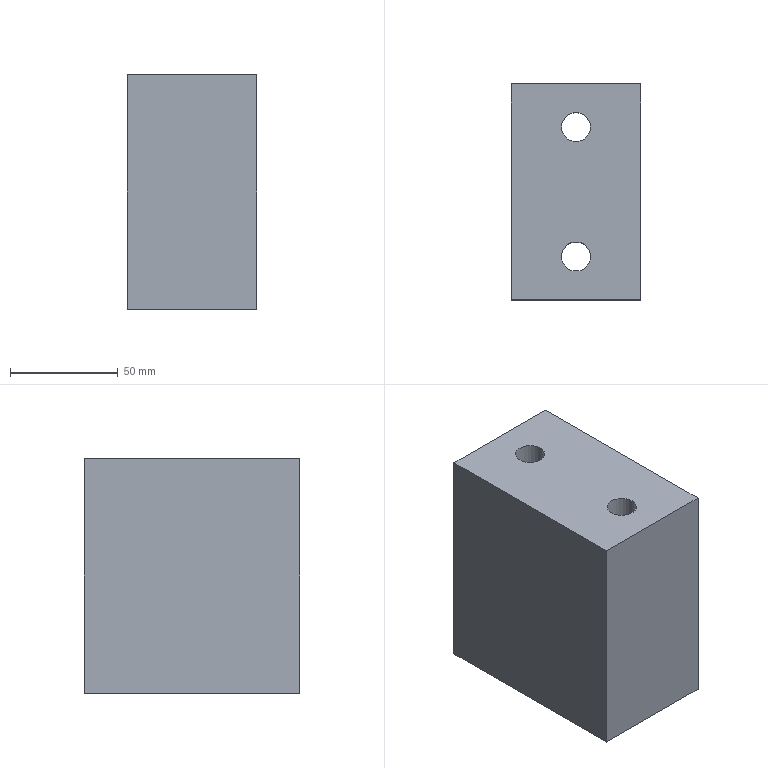Part | NX | features 15 2 | 1 solid | 12 faces | box 60 x 100 x 108.5 mm | volume 596509 mm3 | plane 8 | cylinder 4 | commonest cylinder face diameters 13.5 x2 20 x2
STEP:
#1=CARTESIAN_POINT('',(3961.75,-592.5,61.));
#2=VERTEX_POINT('',#1);
#3=CARTESIAN_POINT('',(3955.,-592.5,61.));
#4=DIRECTION('',(0.,0.,1.));
#5=DIRECTION('',(1.,0.,0.));
#6=AXIS2_PLACEMENT_3D('',#3,#4,#5);
#7=CIRCLE('',#6,6.75);
#8=EDGE_CURVE('',#2,#2,#7,.T.);
#9=ORIENTED_EDGE('',*,*,#8,.T.);
#10=EDGE_LOOP('',(#9));
#11=FACE_BOUND('',#10,.T.);
#12=CARTESIAN_POINT('',(3955.,-602.5,61.));
#13=VERTEX_POINT('',#12);
#14=CARTESIAN_POINT('',(3955.,-592.5,61.));
#15=DIRECTION('',(0.,0.,1.));
#16=DIRECTION('',(0.,-1.,0.));
#17=AXIS2_PLACEMENT_3D('',#14,#15,#16);
#18=CIRCLE('',#17,10.);
#19=EDGE_CURVE('',#13,#13,#18,.T.);
#20=ORIENTED_EDGE('',*,*,#19,.F.);
#21=EDGE_LOOP('',(#20));
#22=FACE_BOUND('',#21,.T.);
#23=CARTESIAN_POINT('',(3959.241,-596.363,61.));
#24=DIRECTION('',(0.,0.,1.));
#25=DIRECTION('',(0.,-1.,0.));
#26=AXIS2_PLACEMENT_3D('',#23,#24,#25);
#27=PLANE('',#26);
#28=ADVANCED_FACE('',(#11,#22),#27,.F.);
#29=ORIENTED_EDGE('',*,*,#19,.T.);
#30=EDGE_LOOP('',(#29));
#31=FACE_BOUND('',#30,.T.);
#32=CARTESIAN_POINT('',(3955.,-602.5,-7.5));
#33=VERTEX_POINT('',#32);
#34=CARTESIAN_POINT('',(3955.,-592.5,-7.5));
#35=DIRECTION('',(0.,0.,-1.));
#36=DIRECTION('',(0.,-1.,0.));
#37=AXIS2_PLACEMENT_3D('',#34,#35,#36);
#38=CIRCLE('',#37,10.);
#39=EDGE_CURVE('',#33,#33,#38,.T.);
#40=ORIENTED_EDGE('',*,*,#39,.T.);
#41=EDGE_LOOP('',(#40));
#42=FACE_BOUND('',#41,.T.);
#43=CARTESIAN_POINT('',(3955.,-592.5,-7.5));
#44=DIRECTION('',(0.,0.,1.));
#45=DIRECTION('',(0.,-1.,0.));
#46=AXIS2_PLACEMENT_3D('',#43,#44,#45);
#47=CYLINDRICAL_SURFACE('',#46,10.);
#48=ADVANCED_FACE('',(#31,#42),#47,.F.);
#49=CARTESIAN_POINT('',(3961.75,-592.5,101.));
#50=VERTEX_POINT('',#49);
#51=CARTESIAN_POINT('',(3955.,-592.5,101.));
#52=DIRECTION('',(0.,0.,1.));
#53=DIRECTION('',(1.,0.,0.));
#54=AXIS2_PLACEMENT_3D('',#51,#52,#53);
#55=CIRCLE('',#54,6.75);
#56=EDGE_CURVE('',#50,#50,#55,.T.);
#57=ORIENTED_EDGE('',*,*,#56,.T.);
#58=EDGE_LOOP('',(#57));
#59=FACE_BOUND('',#58,.T.);
#60=ORIENTED_EDGE('',*,*,#8,.F.);
#61=EDGE_LOOP('',(#60));
#62=FACE_BOUND('',#61,.T.);
#63=CARTESIAN_POINT('',(3955.,-592.5,12.5));
#64=DIRECTION('',(0.,0.,1.));
#65=DIRECTION('',(0.,-1.,0.));
#66=AXIS2_PLACEMENT_3D('',#63,#64,#65);
#67=CYLINDRICAL_SURFACE('',#66,6.75);
#68=ADVANCED_FACE('',(#59,#62),#67,.F.);
#69=CARTESIAN_POINT('',(3961.75,-652.5,61.));
#70=VERTEX_POINT('',#69);
#71=CARTESIAN_POINT('',(3955.,-652.5,61.));
#72=DIRECTION('',(0.,0.,1.));
#73=DIRECTION('',(1.,0.,0.));
#74=AXIS2_PLACEMENT_3D('',#71,#72,#73);
#75=CIRCLE('',#74,6.75);
#76=EDGE_CURVE('',#70,#70,#75,.T.);
#77=ORIENTED_EDGE('',*,*,#76,.T.);
#78=EDGE_LOOP('',(#77));
#79=FACE_BOUND('',#78,.T.);
#80=CARTESIAN_POINT('',(3955.,-662.5,61.));
#81=VERTEX_POINT('',#80);
#82=CARTESIAN_POINT('',(3955.,-652.5,61.));
#83=DIRECTION('',(0.,0.,1.));
#84=DIRECTION('',(0.,-1.,0.));
#85=AXIS2_PLACEMENT_3D('',#82,#83,#84);
#86=CIRCLE('',#85,10.);
#87=EDGE_CURVE('',#81,#81,#86,.T.);
#88=ORIENTED_EDGE('',*,*,#87,.F.);
#89=EDGE_LOOP('',(#88));
#90=FACE_BOUND('',#89,.T.);
#91=CARTESIAN_POINT('',(3959.241,-648.637,61.));
#92=DIRECTION('',(0.,0.,1.));
#93=DIRECTION('',(0.,1.,0.));
#94=AXIS2_PLACEMENT_3D('',#91,#92,#93);
#95=PLANE('',#94);
#96=ADVANCED_FACE('',(#79,#90),#95,.F.);
#97=CARTESIAN_POINT('',(3961.75,-652.5,101.));
#98=VERTEX_POINT('',#97);
#99=CARTESIAN_POINT('',(3955.,-652.5,101.));
#100=DIRECTION('',(0.,0.,1.));
#101=DIRECTION('',(1.,0.,0.));
#102=AXIS2_PLACEMENT_3D('',#99,#100,#101);
#103=CIRCLE('',#102,6.75);
#104=EDGE_CURVE('',#98,#98,#103,.T.);
#105=ORIENTED_EDGE('',*,*,#104,.T.);
#106=EDGE_LOOP('',(#105));
#107=FACE_BOUND('',#106,.T.);
#108=ORIENTED_EDGE('',*,*,#76,.F.);
#109=EDGE_LOOP('',(#108));
#110=FACE_BOUND('',#109,.T.);
#111=CARTESIAN_POINT('',(3955.,-652.5,12.5));
#112=DIRECTION('',(0.,0.,1.));
#113=DIRECTION('',(0.,1.,0.));
#114=AXIS2_PLACEMENT_3D('',#111,#112,#113);
#115=CYLINDRICAL_SURFACE('',#114,6.75);
#116=ADVANCED_FACE('',(#107,#110),#115,.F.);
#117=CARTESIAN_POINT('',(3925.,-572.5,101.));
#118=VERTEX_POINT('',#117);
#119=CARTESIAN_POINT('',(3925.,-572.5,-7.5));
#120=VERTEX_POINT('',#119);
#121=CARTESIAN_POINT('',(3925.,-572.5,48.));
#122=DIRECTION('',(0.,0.,-1.));
#123=VECTOR('',#122,1000.);
#124=LINE('',#121,#123);
#125=EDGE_CURVE('',#118,#120,#124,.T.);
#126=ORIENTED_EDGE('',*,*,#125,.F.);
#127=CARTESIAN_POINT('',(3985.,-572.5,101.));
#128=VERTEX_POINT('',#127);
#129=CARTESIAN_POINT('',(3985.,-572.5,101.));
#130=DIRECTION('',(-1.,0.,0.));
#131=VECTOR('',#130,1000.);
#132=LINE('',#129,#131);
#133=EDGE_CURVE('',#128,#118,#132,.T.);
#134=ORIENTED_EDGE('',*,*,#133,.F.);
#135=CARTESIAN_POINT('',(3985.,-572.5,-7.5));
#136=VERTEX_POINT('',#135);
#137=CARTESIAN_POINT('',(3985.,-572.5,48.));
#138=DIRECTION('',(0.,0.,1.));
#139=VECTOR('',#138,1000.);
#140=LINE('',#137,#139);
#141=EDGE_CURVE('',#136,#128,#140,.T.);
#142=ORIENTED_EDGE('',*,*,#141,.F.);
#143=CARTESIAN_POINT('',(3985.,-572.5,-7.5));
#144=DIRECTION('',(1.,0.,0.));
#145=VECTOR('',#144,1000.);
#146=LINE('',#143,#145);
#147=EDGE_CURVE('',#120,#136,#146,.T.);
#148=ORIENTED_EDGE('',*,*,#147,.F.);
#149=EDGE_LOOP('',(#126,#134,#142,#148));
#150=FACE_BOUND('',#149,.T.);
#151=CARTESIAN_POINT('',(3985.,-572.5,48.));
#152=DIRECTION('',(0.,1.,0.));
#153=DIRECTION('',(0.,0.,-1.));
#154=AXIS2_PLACEMENT_3D('',#151,#152,#153);
#155=PLANE('',#154);
#156=ADVANCED_FACE('',(#150),#155,.T.);
#157=ORIENTED_EDGE('',*,*,#141,.T.);
#158=CARTESIAN_POINT('',(3985.,-672.5,101.));
#159=VERTEX_POINT('',#158);
#160=CARTESIAN_POINT('',(3985.,266.621,101.));
#161=DIRECTION('',(0.,-1.,0.));
#162=VECTOR('',#161,1000.);
#163=LINE('',#160,#162);
#164=EDGE_CURVE('',#128,#159,#163,.T.);
#165=ORIENTED_EDGE('',*,*,#164,.T.);
#166=CARTESIAN_POINT('',(3985.,-672.5,-7.5));
#167=VERTEX_POINT('',#166);
#168=CARTESIAN_POINT('',(3985.,-672.5,48.));
#169=DIRECTION('',(0.,0.,-1.));
#170=VECTOR('',#169,1000.);
#171=LINE('',#168,#170);
#172=EDGE_CURVE('',#159,#167,#171,.T.);
#173=ORIENTED_EDGE('',*,*,#172,.T.);
#174=CARTESIAN_POINT('',(3985.,-642.5,-7.5));
#175=DIRECTION('',(0.,-1.,0.));
#176=VECTOR('',#175,1000.);
#177=LINE('',#174,#176);
#178=EDGE_CURVE('',#136,#167,#177,.T.);
#179=ORIENTED_EDGE('',*,*,#178,.F.);
#180=EDGE_LOOP('',(#157,#165,#173,#179));
#181=FACE_BOUND('',#180,.T.);
#182=CARTESIAN_POINT('',(3985.,-642.5,48.));
#183=DIRECTION('',(1.,0.,0.));
#184=DIRECTION('',(0.,0.,-1.));
#185=AXIS2_PLACEMENT_3D('',#182,#183,#184);
#186=PLANE('',#185);
#187=ADVANCED_FACE('',(#181),#186,.T.);
#188=ORIENTED_EDGE('',*,*,#172,.F.);
#189=CARTESIAN_POINT('',(3925.,-672.5,101.));
#190=VERTEX_POINT('',#189);
#191=CARTESIAN_POINT('',(3600.,-672.5,101.));
#192=DIRECTION('',(-1.,0.,0.));
#193=VECTOR('',#192,1000.);
#194=LINE('',#191,#193);
#195=EDGE_CURVE('',#159,#190,#194,.T.);
#196=ORIENTED_EDGE('',*,*,#195,.T.);
#197=CARTESIAN_POINT('',(3925.,-672.5,-7.5));
#198=VERTEX_POINT('',#197);
#199=CARTESIAN_POINT('',(3925.,-672.5,48.));
#200=DIRECTION('',(0.,0.,1.));
#201=VECTOR('',#200,1000.);
#202=LINE('',#199,#201);
#203=EDGE_CURVE('',#198,#190,#202,.T.);
#204=ORIENTED_EDGE('',*,*,#203,.F.);
#205=CARTESIAN_POINT('',(3985.,-672.5,-7.5));
#206=DIRECTION('',(-1.,0.,0.));
#207=VECTOR('',#206,1000.);
#208=LINE('',#205,#207);
#209=EDGE_CURVE('',#167,#198,#208,.T.);
#210=ORIENTED_EDGE('',*,*,#209,.F.);
#211=EDGE_LOOP('',(#188,#196,#204,#210));
#212=FACE_BOUND('',#211,.T.);
#213=CARTESIAN_POINT('',(3985.,-672.5,48.));
#214=DIRECTION('',(0.,-1.,0.));
#215=DIRECTION('',(0.,0.,1.));
#216=AXIS2_PLACEMENT_3D('',#213,#214,#215);
#217=PLANE('',#216);
#218=ADVANCED_FACE('',(#212),#217,.T.);
#219=ORIENTED_EDGE('',*,*,#203,.T.);
#220=CARTESIAN_POINT('',(3925.,266.621,101.));
#221=DIRECTION('',(0.,1.,0.));
#222=VECTOR('',#221,1000.);
#223=LINE('',#220,#222);
#224=EDGE_CURVE('',#190,#118,#223,.T.);
#225=ORIENTED_EDGE('',*,*,#224,.T.);
#226=ORIENTED_EDGE('',*,*,#125,.T.);
#227=CARTESIAN_POINT('',(3925.,-642.5,-7.5));
#228=DIRECTION('',(0.,1.,0.));
#229=VECTOR('',#228,1000.);
#230=LINE('',#227,#229);
#231=EDGE_CURVE('',#198,#120,#230,.T.);
#232=ORIENTED_EDGE('',*,*,#231,.F.);
#233=EDGE_LOOP('',(#219,#225,#226,#232));
#234=FACE_BOUND('',#233,.T.);
#235=CARTESIAN_POINT('',(3925.,-642.5,48.));
#236=DIRECTION('',(-1.,0.,0.));
#237=DIRECTION('',(0.,0.,1.));
#238=AXIS2_PLACEMENT_3D('',#235,#236,#237);
#239=PLANE('',#238);
#240=ADVANCED_FACE('',(#234),#239,.T.);
#241=ORIENTED_EDGE('',*,*,#87,.T.);
#242=EDGE_LOOP('',(#241));
#243=FACE_BOUND('',#242,.T.);
#244=CARTESIAN_POINT('',(3955.,-642.5,-7.5));
#245=VERTEX_POINT('',#244);
#246=CARTESIAN_POINT('',(3955.,-652.5,-7.5));
#247=DIRECTION('',(0.,0.,-1.));
#248=DIRECTION('',(0.,1.,0.));
#249=AXIS2_PLACEMENT_3D('',#246,#247,#248);
#250=CIRCLE('',#249,10.);
#251=EDGE_CURVE('',#245,#245,#250,.T.);
#252=ORIENTED_EDGE('',*,*,#251,.T.);
#253=EDGE_LOOP('',(#252));
#254=FACE_BOUND('',#253,.T.);
#255=CARTESIAN_POINT('',(3955.,-652.5,-7.5));
#256=DIRECTION('',(0.,0.,1.));
#257=DIRECTION('',(0.,1.,0.));
#258=AXIS2_PLACEMENT_3D('',#255,#256,#257);
#259=CYLINDRICAL_SURFACE('',#258,10.);
#260=ADVANCED_FACE('',(#243,#254),#259,.F.);
#261=ORIENTED_EDGE('',*,*,#39,.F.);
#262=EDGE_LOOP('',(#261));
#263=FACE_BOUND('',#262,.T.);
#264=ORIENTED_EDGE('',*,*,#251,.F.);
#265=EDGE_LOOP('',(#264));
#266=FACE_BOUND('',#265,.T.);
#267=ORIENTED_EDGE('',*,*,#231,.T.);
#268=ORIENTED_EDGE('',*,*,#147,.T.);
#269=ORIENTED_EDGE('',*,*,#178,.T.);
#270=ORIENTED_EDGE('',*,*,#209,.T.);
#271=EDGE_LOOP('',(#267,#268,#269,#270));
#272=FACE_BOUND('',#271,.T.);
#273=CARTESIAN_POINT('',(3985.,-572.5,-7.5));
#274=DIRECTION('',(0.,0.,-1.));
#275=DIRECTION('',(0.,-1.,0.));
#276=AXIS2_PLACEMENT_3D('',#273,#274,#275);
#277=PLANE('',#276);
#278=ADVANCED_FACE('',(#263,#266,#272),#277,.T.);
#279=ORIENTED_EDGE('',*,*,#56,.F.);
#280=EDGE_LOOP('',(#279));
#281=FACE_BOUND('',#280,.T.);
#282=ORIENTED_EDGE('',*,*,#195,.F.);
#283=ORIENTED_EDGE('',*,*,#164,.F.);
#284=ORIENTED_EDGE('',*,*,#133,.T.);
#285=ORIENTED_EDGE('',*,*,#224,.F.);
#286=EDGE_LOOP('',(#282,#283,#284,#285));
#287=FACE_BOUND('',#286,.T.);
#288=ORIENTED_EDGE('',*,*,#104,.F.);
#289=EDGE_LOOP('',(#288));
#290=FACE_BOUND('',#289,.T.);
#291=CARTESIAN_POINT('',(3600.,266.621,101.));
#292=DIRECTION('',(0.,0.,1.));
#293=DIRECTION('',(0.,1.,0.));
#294=AXIS2_PLACEMENT_3D('',#291,#292,#293);
#295=PLANE('',#294);
#296=ADVANCED_FACE('',(#281,#287,#290),#295,.T.);
#297=CLOSED_SHELL('',(#28,#48,#68,#96,#116,#156,#187,#218,#240,#260,#278,#296));
#298=MANIFOLD_SOLID_BREP('',#297);
#299=(LENGTH_UNIT()NAMED_UNIT(*)SI_UNIT(.MILLI.,.METRE.));
#300=UNCERTAINTY_MEASURE_WITH_UNIT(LENGTH_MEASURE(0.00001),#299,'','');
#301=(NAMED_UNIT(*)PLANE_ANGLE_UNIT()SI_UNIT($,.RADIAN.));
#302=(NAMED_UNIT(*)SI_UNIT($,.STERADIAN.)SOLID_ANGLE_UNIT());
#303=(GEOMETRIC_REPRESENTATION_CONTEXT(3)GLOBAL_UNCERTAINTY_ASSIGNED_CONTEXT((#300))GLOBAL_UNIT_ASSIGNED_CONTEXT((#299,#301,#302))REPRESENTATION_CONTEXT('',''));
#304=ADVANCED_BREP_SHAPE_REPRESENTATION('',(#298),#303);